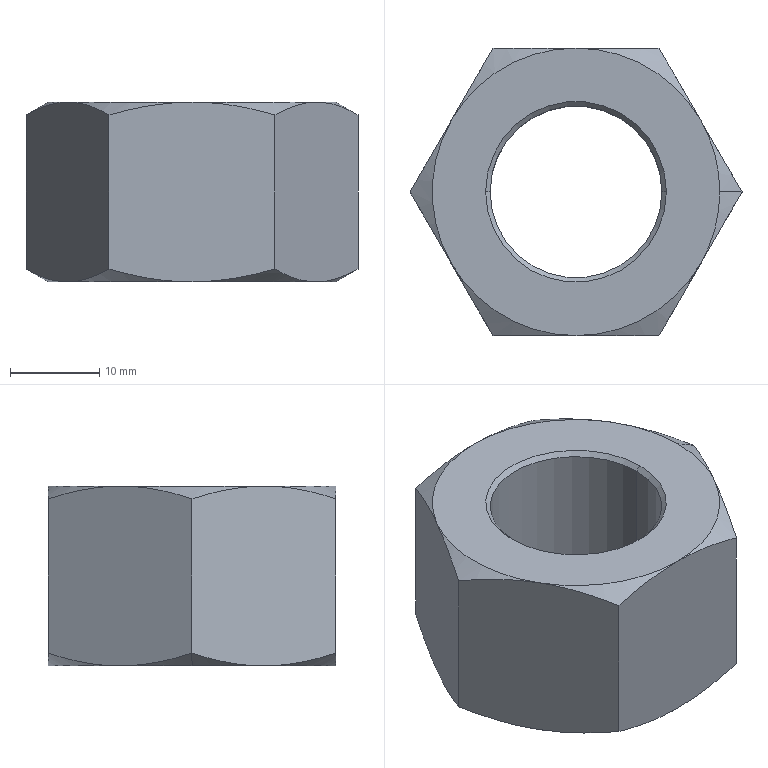Part | SolidWorks | features Cut 2, Chamfer 1, Extrusion 1 | 1 solid | 28 faces | box 37.3 x 32.303 x 20.2 mm | volume 12259 mm3 | cone 18 | plane 8 | cylinder 2 | commonest cylinder face diameters 19.294 x2
STEP:
#1=CARTESIAN_POINT('',(-9.647,0.,19.695));
#2=VERTEX_POINT('',#1);
#3=CARTESIAN_POINT('',(9.647,0.,19.695));
#4=VERTEX_POINT('',#3);
#5=CARTESIAN_POINT('',(0.,0.,19.695));
#6=DIRECTION('',(0.,0.,1.));
#7=DIRECTION('',(-1.,0.,0.));
#8=AXIS2_PLACEMENT_3D('',#5,#6,#7);
#9=CIRCLE('',#8,9.647);
#10=EDGE_CURVE('',#2,#4,#9,.T.);
#11=ORIENTED_EDGE('',*,*,#10,.F.);
#12=CARTESIAN_POINT('',(-10.152,0.,20.2));
#13=VERTEX_POINT('',#12);
#14=CARTESIAN_POINT('',(-9.647,0.,19.695));
#15=DIRECTION('',(-0.7071,0.,0.7071));
#16=VECTOR('',#15,1000.);
#17=LINE('',#14,#16);
#18=EDGE_CURVE('',#2,#13,#17,.T.);
#19=ORIENTED_EDGE('',*,*,#18,.T.);
#20=CARTESIAN_POINT('',(10.152,0.,20.2));
#21=VERTEX_POINT('',#20);
#22=CARTESIAN_POINT('',(0.,0.,20.2));
#23=DIRECTION('',(0.,0.,-1.));
#24=DIRECTION('',(-1.,0.,0.));
#25=AXIS2_PLACEMENT_3D('',#22,#23,#24);
#26=CIRCLE('',#25,10.152);
#27=EDGE_CURVE('',#21,#13,#26,.T.);
#28=ORIENTED_EDGE('',*,*,#27,.F.);
#29=CARTESIAN_POINT('',(9.647,0.,19.695));
#30=DIRECTION('',(0.7071,0.,0.7071));
#31=VECTOR('',#30,1000.);
#32=LINE('',#29,#31);
#33=EDGE_CURVE('',#4,#21,#32,.T.);
#34=ORIENTED_EDGE('',*,*,#33,.F.);
#35=EDGE_LOOP('',(#11,#19,#28,#34));
#36=FACE_OUTER_BOUND('',#35,.T.);
#37=CARTESIAN_POINT('',(0.,0.,19.695));
#38=DIRECTION('',(0.,0.,1.));
#39=DIRECTION('',(1.,0.,0.));
#40=AXIS2_PLACEMENT_3D('',#37,#38,#39);
#41=CONICAL_SURFACE('',#40,9.647,0.7854);
#42=ADVANCED_FACE('',(#36),#41,.F.);
#43=CARTESIAN_POINT('',(9.647,0.,0.505));
#44=VERTEX_POINT('',#43);
#45=CARTESIAN_POINT('',(-9.647,0.,0.505));
#46=VERTEX_POINT('',#45);
#47=CARTESIAN_POINT('',(0.,0.,0.505));
#48=DIRECTION('',(0.,0.,-1.));
#49=DIRECTION('',(-1.,0.,0.));
#50=AXIS2_PLACEMENT_3D('',#47,#48,#49);
#51=CIRCLE('',#50,9.647);
#52=EDGE_CURVE('',#44,#46,#51,.T.);
#53=ORIENTED_EDGE('',*,*,#52,.F.);
#54=CARTESIAN_POINT('',(10.152,0.,0.));
#55=VERTEX_POINT('',#54);
#56=CARTESIAN_POINT('',(10.152,0.,0.));
#57=DIRECTION('',(0.7071,0.,-0.7071));
#58=VECTOR('',#57,1000.);
#59=LINE('',#56,#58);
#60=EDGE_CURVE('',#44,#55,#59,.T.);
#61=ORIENTED_EDGE('',*,*,#60,.T.);
#62=CARTESIAN_POINT('',(-10.152,0.,0.));
#63=VERTEX_POINT('',#62);
#64=CARTESIAN_POINT('',(0.,0.,0.));
#65=DIRECTION('',(0.,0.,1.));
#66=DIRECTION('',(-1.,0.,0.));
#67=AXIS2_PLACEMENT_3D('',#64,#65,#66);
#68=CIRCLE('',#67,10.152);
#69=EDGE_CURVE('',#63,#55,#68,.T.);
#70=ORIENTED_EDGE('',*,*,#69,.F.);
#71=CARTESIAN_POINT('',(-10.152,0.,0.));
#72=DIRECTION('',(-0.7071,0.,-0.7071));
#73=VECTOR('',#72,1000.);
#74=LINE('',#71,#73);
#75=EDGE_CURVE('',#46,#63,#74,.T.);
#76=ORIENTED_EDGE('',*,*,#75,.F.);
#77=EDGE_LOOP('',(#53,#61,#70,#76));
#78=FACE_OUTER_BOUND('',#77,.T.);
#79=CARTESIAN_POINT('',(0.,0.,0.));
#80=DIRECTION('',(0.,0.,-1.));
#81=DIRECTION('',(-1.,0.,0.));
#82=AXIS2_PLACEMENT_3D('',#79,#80,#81);
#83=CONICAL_SURFACE('',#82,10.152,0.7854);
#84=ADVANCED_FACE('',(#78),#83,.F.);
#85=CARTESIAN_POINT('',(13.988,8.076,20.2));
#86=VERTEX_POINT('',#85);
#87=CARTESIAN_POINT('',(16.151,0.,20.2));
#88=VERTEX_POINT('',#87);
#89=CARTESIAN_POINT('',(0.,0.,20.2));
#90=DIRECTION('',(0.,0.,-1.));
#91=DIRECTION('',(-1.,0.,0.));
#92=AXIS2_PLACEMENT_3D('',#89,#90,#91);
#93=CIRCLE('',#92,16.151);
#94=EDGE_CURVE('',#86,#88,#93,.T.);
#95=ORIENTED_EDGE('',*,*,#94,.T.);
#96=CARTESIAN_POINT('',(18.65,0.,18.757));
#97=VERTEX_POINT('',#96);
#98=CARTESIAN_POINT('',(16.151,0.,20.2));
#99=DIRECTION('',(0.866,0.,-0.5));
#100=VECTOR('',#99,1000.);
#101=LINE('',#98,#100);
#102=EDGE_CURVE('',#88,#97,#101,.T.);
#103=ORIENTED_EDGE('',*,*,#102,.T.);
#104=CARTESIAN_POINT('',(18.65,0.,18.757));
#105=CARTESIAN_POINT('',(17.887,1.321,19.198));
#106=CARTESIAN_POINT('',(17.119,2.652,19.561));
#107=CARTESIAN_POINT('',(15.566,5.341,20.063));
#108=CARTESIAN_POINT('',(14.782,6.7,20.2));
#109=CARTESIAN_POINT('',(13.988,8.076,20.2));
#110=B_SPLINE_CURVE_WITH_KNOTS('',3,(#104,#105,#106,#107,#108,#109),.UNSPECIFIED.,.F.,.F.,(4,2,4),(0.000000238,0.004718,0.009436),.UNSPECIFIED.);
#111=EDGE_CURVE('',#97,#86,#110,.T.);
#112=ORIENTED_EDGE('',*,*,#111,.T.);
#113=EDGE_LOOP('',(#95,#103,#112));
#114=FACE_OUTER_BOUND('',#113,.T.);
#115=CARTESIAN_POINT('',(0.,0.,20.2));
#116=DIRECTION('',(0.,0.,-1.));
#117=DIRECTION('',(1.,0.,0.));
#118=AXIS2_PLACEMENT_3D('',#115,#116,#117);
#119=CONICAL_SURFACE('',#118,16.151,1.047);
#120=ADVANCED_FACE('',(#114),#119,.T.);
#121=CARTESIAN_POINT('',(-16.151,0.,0.));
#122=VERTEX_POINT('',#121);
#123=CARTESIAN_POINT('',(-13.988,8.076,0.));
#124=VERTEX_POINT('',#123);
#125=CARTESIAN_POINT('',(0.,0.,0.));
#126=DIRECTION('',(0.,0.,-1.));
#127=DIRECTION('',(-1.,0.,0.));
#128=AXIS2_PLACEMENT_3D('',#125,#126,#127);
#129=CIRCLE('',#128,16.151);
#130=EDGE_CURVE('',#122,#124,#129,.T.);
#131=ORIENTED_EDGE('',*,*,#130,.F.);
#132=CARTESIAN_POINT('',(-18.65,0.,1.443));
#133=VERTEX_POINT('',#132);
#134=CARTESIAN_POINT('',(-16.151,0.,0.));
#135=DIRECTION('',(-0.866,0.,0.5));
#136=VECTOR('',#135,1000.);
#137=LINE('',#134,#136);
#138=EDGE_CURVE('',#122,#133,#137,.T.);
#139=ORIENTED_EDGE('',*,*,#138,.T.);
#140=CARTESIAN_POINT('',(-18.65,0.,1.443));
#141=CARTESIAN_POINT('',(-17.887,1.321,1.002));
#142=CARTESIAN_POINT('',(-17.119,2.652,0.6394));
#143=CARTESIAN_POINT('',(-15.566,5.341,0.1375));
#144=CARTESIAN_POINT('',(-14.782,6.7,0.));
#145=CARTESIAN_POINT('',(-13.988,8.076,0.));
#146=B_SPLINE_CURVE_WITH_KNOTS('',3,(#140,#141,#142,#143,#144,#145),.UNSPECIFIED.,.F.,.F.,(4,2,4),(0.000000238,0.004718,0.009436),.UNSPECIFIED.);
#147=EDGE_CURVE('',#133,#124,#146,.T.);
#148=ORIENTED_EDGE('',*,*,#147,.T.);
#149=EDGE_LOOP('',(#131,#139,#148));
#150=FACE_OUTER_BOUND('',#149,.T.);
#151=CARTESIAN_POINT('',(0.,0.,0.));
#152=DIRECTION('',(0.,0.,1.));
#153=DIRECTION('',(-1.,0.,0.));
#154=AXIS2_PLACEMENT_3D('',#151,#152,#153);
#155=CONICAL_SURFACE('',#154,16.151,1.047);
#156=ADVANCED_FACE('',(#150),#155,.T.);
#157=ORIENTED_EDGE('',*,*,#10,.T.);
#158=CARTESIAN_POINT('',(9.647,0.,20.2));
#159=DIRECTION('',(0.,0.,-1.));
#160=VECTOR('',#159,1000.);
#161=LINE('',#158,#160);
#162=EDGE_CURVE('',#4,#44,#161,.T.);
#163=ORIENTED_EDGE('',*,*,#162,.T.);
#164=ORIENTED_EDGE('',*,*,#52,.T.);
#165=CARTESIAN_POINT('',(-9.647,0.,20.2));
#166=DIRECTION('',(0.,0.,-1.));
#167=VECTOR('',#166,1000.);
#168=LINE('',#165,#167);
#169=EDGE_CURVE('',#2,#46,#168,.T.);
#170=ORIENTED_EDGE('',*,*,#169,.F.);
#171=EDGE_LOOP('',(#157,#163,#164,#170));
#172=FACE_OUTER_BOUND('',#171,.T.);
#173=CARTESIAN_POINT('',(0.,0.,20.2));
#174=DIRECTION('',(0.,0.,-1.));
#175=DIRECTION('',(-1.,0.,0.));
#176=AXIS2_PLACEMENT_3D('',#173,#174,#175);
#177=CYLINDRICAL_SURFACE('',#176,9.647);
#178=ADVANCED_FACE('',(#172),#177,.F.);
#179=ORIENTED_EDGE('',*,*,#111,.F.);
#180=CARTESIAN_POINT('',(18.65,0.,1.443));
#181=VERTEX_POINT('',#180);
#182=CARTESIAN_POINT('',(18.65,0.,20.2));
#183=DIRECTION('',(0.,0.,-1.));
#184=VECTOR('',#183,1000.);
#185=LINE('',#182,#184);
#186=EDGE_CURVE('',#97,#181,#185,.T.);
#187=ORIENTED_EDGE('',*,*,#186,.T.);
#188=CARTESIAN_POINT('',(13.988,8.076,0.));
#189=VERTEX_POINT('',#188);
#190=CARTESIAN_POINT('',(13.988,8.076,0.));
#191=CARTESIAN_POINT('',(14.383,7.39,0.));
#192=CARTESIAN_POINT('',(14.781,6.702,0.0341));
#193=CARTESIAN_POINT('',(15.567,5.34,0.166));
#194=CARTESIAN_POINT('',(15.957,4.664,0.2638));
#195=CARTESIAN_POINT('',(17.122,2.647,0.6407));
#196=CARTESIAN_POINT('',(17.889,1.318,1.003));
#197=CARTESIAN_POINT('',(18.65,0.,1.443));
#198=B_SPLINE_CURVE_WITH_KNOTS('',3,(#190,#191,#192,#193,#194,#195,#196,#197),.UNSPECIFIED.,.F.,.F.,(4,2,2,4),(0.009436,0.01179,0.01414,0.01884),.UNSPECIFIED.);
#199=EDGE_CURVE('',#189,#181,#198,.T.);
#200=ORIENTED_EDGE('',*,*,#199,.F.);
#201=CARTESIAN_POINT('',(9.325,16.151,1.443));
#202=VERTEX_POINT('',#201);
#203=CARTESIAN_POINT('',(9.325,16.151,1.443));
#204=CARTESIAN_POINT('',(10.088,14.83,1.002));
#205=CARTESIAN_POINT('',(10.856,13.5,0.6394));
#206=CARTESIAN_POINT('',(12.409,10.81,0.1375));
#207=CARTESIAN_POINT('',(13.193,9.452,0.));
#208=CARTESIAN_POINT('',(13.988,8.076,0.));
#209=B_SPLINE_CURVE_WITH_KNOTS('',3,(#203,#204,#205,#206,#207,#208),.UNSPECIFIED.,.F.,.F.,(4,2,4),(0.000000238,0.004718,0.009436),.UNSPECIFIED.);
#210=EDGE_CURVE('',#202,#189,#209,.T.);
#211=ORIENTED_EDGE('',*,*,#210,.F.);
#212=CARTESIAN_POINT('',(9.325,16.151,18.757));
#213=VERTEX_POINT('',#212);
#214=CARTESIAN_POINT('',(9.325,16.151,20.2));
#215=DIRECTION('',(0.,0.,-1.));
#216=VECTOR('',#215,1000.);
#217=LINE('',#214,#216);
#218=EDGE_CURVE('',#213,#202,#217,.T.);
#219=ORIENTED_EDGE('',*,*,#218,.F.);
#220=CARTESIAN_POINT('',(13.988,8.076,20.2));
#221=CARTESIAN_POINT('',(13.592,8.761,20.2));
#222=CARTESIAN_POINT('',(13.194,9.449,20.166));
#223=CARTESIAN_POINT('',(12.408,10.811,20.034));
#224=CARTESIAN_POINT('',(12.018,11.488,19.936));
#225=CARTESIAN_POINT('',(10.853,13.505,19.559));
#226=CARTESIAN_POINT('',(10.086,14.834,19.197));
#227=CARTESIAN_POINT('',(9.325,16.151,18.757));
#228=B_SPLINE_CURVE_WITH_KNOTS('',3,(#220,#221,#222,#223,#224,#225,#226,#227),.UNSPECIFIED.,.F.,.F.,(4,2,2,4),(0.009436,0.01179,0.01414,0.01884),.UNSPECIFIED.);
#229=EDGE_CURVE('',#86,#213,#228,.T.);
#230=ORIENTED_EDGE('',*,*,#229,.F.);
#231=EDGE_LOOP('',(#179,#187,#200,#211,#219,#230));
#232=FACE_OUTER_BOUND('',#231,.T.);
#233=CARTESIAN_POINT('',(18.65,0.,20.2));
#234=DIRECTION('',(-0.866,-0.5,0.));
#235=DIRECTION('',(0.5,-0.866,0.));
#236=AXIS2_PLACEMENT_3D('',#233,#234,#235);
#237=PLANE('',#236);
#238=ADVANCED_FACE('',(#232),#237,.F.);
#239=CARTESIAN_POINT('',(0.,16.151,20.2));
#240=VERTEX_POINT('',#239);
#241=CARTESIAN_POINT('',(9.325,16.151,18.757));
#242=CARTESIAN_POINT('',(7.817,16.151,19.193));
#243=CARTESIAN_POINT('',(6.29,16.151,19.555));
#244=CARTESIAN_POINT('',(3.955,16.151,19.934));
#245=CARTESIAN_POINT('',(3.17,16.151,20.033));
#246=CARTESIAN_POINT('',(1.582,16.151,20.166));
#247=CARTESIAN_POINT('',(0.7891,16.151,20.2));
#248=CARTESIAN_POINT('',(0.,16.151,20.2));
#249=B_SPLINE_CURVE_WITH_KNOTS('',3,(#241,#242,#243,#244,#245,#246,#247,#248),.UNSPECIFIED.,.F.,.F.,(4,2,2,4),(0.05347,0.05819,0.06055,0.06291),.UNSPECIFIED.);
#250=EDGE_CURVE('',#213,#240,#249,.T.);
#251=ORIENTED_EDGE('',*,*,#250,.F.);
#252=ORIENTED_EDGE('',*,*,#218,.T.);
#253=CARTESIAN_POINT('',(0.,16.151,0.));
#254=VERTEX_POINT('',#253);
#255=CARTESIAN_POINT('',(0.,16.151,0.));
#256=CARTESIAN_POINT('',(0.7891,16.151,0.));
#257=CARTESIAN_POINT('',(1.582,16.151,0.03365));
#258=CARTESIAN_POINT('',(3.17,16.151,0.1671));
#259=CARTESIAN_POINT('',(3.955,16.151,0.2658));
#260=CARTESIAN_POINT('',(6.29,16.151,0.6449));
#261=CARTESIAN_POINT('',(7.817,16.151,1.007));
#262=CARTESIAN_POINT('',(9.325,16.151,1.443));
#263=B_SPLINE_CURVE_WITH_KNOTS('',3,(#255,#256,#257,#258,#259,#260,#261,#262),.UNSPECIFIED.,.F.,.F.,(4,2,2,4),(0.02654,0.0289,0.03126,0.03599),.UNSPECIFIED.);
#264=EDGE_CURVE('',#254,#202,#263,.T.);
#265=ORIENTED_EDGE('',*,*,#264,.F.);
#266=CARTESIAN_POINT('',(-9.325,16.151,1.443));
#267=VERTEX_POINT('',#266);
#268=CARTESIAN_POINT('',(-9.325,16.151,1.443));
#269=CARTESIAN_POINT('',(-8.566,16.151,1.223));
#270=CARTESIAN_POINT('',(-7.799,16.151,1.022));
#271=CARTESIAN_POINT('',(-6.252,16.151,0.6658));
#272=CARTESIAN_POINT('',(-5.476,16.151,0.512));
#273=CARTESIAN_POINT('',(-3.143,16.151,0.1357));
#274=CARTESIAN_POINT('',(-1.577,16.151,0.));
#275=CARTESIAN_POINT('',(0.,16.151,0.));
#276=B_SPLINE_CURVE_WITH_KNOTS('',3,(#268,#269,#270,#271,#272,#273,#274,#275),.UNSPECIFIED.,.F.,.F.,(4,2,2,4),(0.0171,0.01946,0.02182,0.02654),.UNSPECIFIED.);
#277=EDGE_CURVE('',#267,#254,#276,.T.);
#278=ORIENTED_EDGE('',*,*,#277,.F.);
#279=CARTESIAN_POINT('',(-9.325,16.151,18.757));
#280=VERTEX_POINT('',#279);
#281=CARTESIAN_POINT('',(-9.325,16.151,20.2));
#282=DIRECTION('',(0.,0.,-1.));
#283=VECTOR('',#282,1000.);
#284=LINE('',#281,#283);
#285=EDGE_CURVE('',#280,#267,#284,.T.);
#286=ORIENTED_EDGE('',*,*,#285,.F.);
#287=CARTESIAN_POINT('',(0.,16.151,20.2));
#288=CARTESIAN_POINT('',(-1.577,16.151,20.2));
#289=CARTESIAN_POINT('',(-3.143,16.151,20.064));
#290=CARTESIAN_POINT('',(-5.476,16.151,19.688));
#291=CARTESIAN_POINT('',(-6.252,16.151,19.534));
#292=CARTESIAN_POINT('',(-7.799,16.151,19.178));
#293=CARTESIAN_POINT('',(-8.566,16.151,18.977));
#294=CARTESIAN_POINT('',(-9.325,16.151,18.757));
#295=B_SPLINE_CURVE_WITH_KNOTS('',3,(#287,#288,#289,#290,#291,#292,#293,#294),.UNSPECIFIED.,.F.,.F.,(4,2,2,4),(0.06291,0.06763,0.06999,0.07235),.UNSPECIFIED.);
#296=EDGE_CURVE('',#240,#280,#295,.T.);
#297=ORIENTED_EDGE('',*,*,#296,.F.);
#298=EDGE_LOOP('',(#251,#252,#265,#278,#286,#297));
#299=FACE_OUTER_BOUND('',#298,.T.);
#300=CARTESIAN_POINT('',(9.325,16.151,20.2));
#301=DIRECTION('',(0.,-1.,0.));
#302=DIRECTION('',(1.,0.,0.));
#303=AXIS2_PLACEMENT_3D('',#300,#301,#302);
#304=PLANE('',#303);
#305=ADVANCED_FACE('',(#299),#304,.F.);
#306=CARTESIAN_POINT('',(-13.988,8.076,20.2));
#307=VERTEX_POINT('',#306);
#308=CARTESIAN_POINT('',(-9.325,16.151,18.757));
#309=CARTESIAN_POINT('',(-10.088,14.83,19.198));
#310=CARTESIAN_POINT('',(-10.856,13.5,19.561));
#311=CARTESIAN_POINT('',(-12.409,10.81,20.063));
#312=CARTESIAN_POINT('',(-13.193,9.452,20.2));
#313=CARTESIAN_POINT('',(-13.988,8.076,20.2));
#314=B_SPLINE_CURVE_WITH_KNOTS('',3,(#308,#309,#310,#311,#312,#313),.UNSPECIFIED.,.F.,.F.,(4,2,4),(0.000000238,0.004718,0.009436),.UNSPECIFIED.);
#315=EDGE_CURVE('',#280,#307,#314,.T.);
#316=ORIENTED_EDGE('',*,*,#315,.F.);
#317=ORIENTED_EDGE('',*,*,#285,.T.);
#318=CARTESIAN_POINT('',(-13.988,8.076,0.));
#319=CARTESIAN_POINT('',(-13.592,8.761,0.));
#320=CARTESIAN_POINT('',(-13.194,9.449,0.0341));
#321=CARTESIAN_POINT('',(-12.408,10.811,0.166));
#322=CARTESIAN_POINT('',(-12.018,11.488,0.2638));
#323=CARTESIAN_POINT('',(-10.853,13.505,0.6407));
#324=CARTESIAN_POINT('',(-10.086,14.834,1.003));
#325=CARTESIAN_POINT('',(-9.325,16.151,1.443));
#326=B_SPLINE_CURVE_WITH_KNOTS('',3,(#318,#319,#320,#321,#322,#323,#324,#325),.UNSPECIFIED.,.F.,.F.,(4,2,2,4),(0.009436,0.01179,0.01414,0.01884),.UNSPECIFIED.);
#327=EDGE_CURVE('',#124,#267,#326,.T.);
#328=ORIENTED_EDGE('',*,*,#327,.F.);
#329=ORIENTED_EDGE('',*,*,#147,.F.);
#330=CARTESIAN_POINT('',(-18.65,0.,18.757));
#331=VERTEX_POINT('',#330);
#332=CARTESIAN_POINT('',(-18.65,0.,20.2));
#333=DIRECTION('',(0.,0.,-1.));
#334=VECTOR('',#333,1000.);
#335=LINE('',#332,#334);
#336=EDGE_CURVE('',#331,#133,#335,.T.);
#337=ORIENTED_EDGE('',*,*,#336,.F.);
#338=CARTESIAN_POINT('',(-13.988,8.076,20.2));
#339=CARTESIAN_POINT('',(-14.383,7.39,20.2));
#340=CARTESIAN_POINT('',(-14.781,6.702,20.166));
#341=CARTESIAN_POINT('',(-15.567,5.34,20.034));
#342=CARTESIAN_POINT('',(-15.957,4.664,19.936));
#343=CARTESIAN_POINT('',(-17.122,2.647,19.559));
#344=CARTESIAN_POINT('',(-17.889,1.318,19.197));
#345=CARTESIAN_POINT('',(-18.65,0.,18.757));
#346=B_SPLINE_CURVE_WITH_KNOTS('',3,(#338,#339,#340,#341,#342,#343,#344,#345),.UNSPECIFIED.,.F.,.F.,(4,2,2,4),(0.009436,0.01179,0.01414,0.01884),.UNSPECIFIED.);
#347=EDGE_CURVE('',#307,#331,#346,.T.);
#348=ORIENTED_EDGE('',*,*,#347,.F.);
#349=EDGE_LOOP('',(#316,#317,#328,#329,#337,#348));
#350=FACE_OUTER_BOUND('',#349,.T.);
#351=CARTESIAN_POINT('',(-9.325,16.151,20.2));
#352=DIRECTION('',(0.866,-0.5,0.));
#353=DIRECTION('',(0.5,0.866,0.));
#354=AXIS2_PLACEMENT_3D('',#351,#352,#353);
#355=PLANE('',#354);
#356=ADVANCED_FACE('',(#350),#355,.F.);
#357=CARTESIAN_POINT('',(-13.988,-8.076,20.2));
#358=VERTEX_POINT('',#357);
#359=CARTESIAN_POINT('',(-18.65,0.,18.757));
#360=CARTESIAN_POINT('',(-17.887,-1.321,19.198));
#361=CARTESIAN_POINT('',(-17.119,-2.652,19.561));
#362=CARTESIAN_POINT('',(-15.566,-5.341,20.063));
#363=CARTESIAN_POINT('',(-14.782,-6.7,20.2));
#364=CARTESIAN_POINT('',(-13.988,-8.076,20.2));
#365=B_SPLINE_CURVE_WITH_KNOTS('',3,(#359,#360,#361,#362,#363,#364),.UNSPECIFIED.,.F.,.F.,(4,2,4),(0.000000238,0.004718,0.009436),.UNSPECIFIED.);
#366=EDGE_CURVE('',#331,#358,#365,.T.);
#367=ORIENTED_EDGE('',*,*,#366,.F.);
#368=ORIENTED_EDGE('',*,*,#336,.T.);
#369=CARTESIAN_POINT('',(-13.987,-8.076,0.));
#370=VERTEX_POINT('',#369);
#371=CARTESIAN_POINT('',(-13.987,-8.076,0.));
#372=CARTESIAN_POINT('',(-14.383,-7.39,0.));
#373=CARTESIAN_POINT('',(-14.781,-6.702,0.0341));
#374=CARTESIAN_POINT('',(-15.567,-5.34,0.166));
#375=CARTESIAN_POINT('',(-15.957,-4.664,0.2638));
#376=CARTESIAN_POINT('',(-17.122,-2.647,0.6407));
#377=CARTESIAN_POINT('',(-17.889,-1.318,1.003));
#378=CARTESIAN_POINT('',(-18.65,0.,1.443));
#379=B_SPLINE_CURVE_WITH_KNOTS('',3,(#371,#372,#373,#374,#375,#376,#377,#378),.UNSPECIFIED.,.F.,.F.,(4,2,2,4),(0.009436,0.01179,0.01414,0.01884),.UNSPECIFIED.);
#380=EDGE_CURVE('',#370,#133,#379,.T.);
#381=ORIENTED_EDGE('',*,*,#380,.F.);
#382=CARTESIAN_POINT('',(-9.325,-16.151,1.443));
#383=VERTEX_POINT('',#382);
#384=CARTESIAN_POINT('',(-9.325,-16.151,1.443));
#385=CARTESIAN_POINT('',(-10.088,-14.83,1.002));
#386=CARTESIAN_POINT('',(-10.856,-13.5,0.6394));
#387=CARTESIAN_POINT('',(-12.409,-10.81,0.1375));
#388=CARTESIAN_POINT('',(-13.193,-9.452,0.));
#389=CARTESIAN_POINT('',(-13.987,-8.076,0.));
#390=B_SPLINE_CURVE_WITH_KNOTS('',3,(#384,#385,#386,#387,#388,#389),.UNSPECIFIED.,.F.,.F.,(4,2,4),(0.000000238,0.004718,0.009436),.UNSPECIFIED.);
#391=EDGE_CURVE('',#383,#370,#390,.T.);
#392=ORIENTED_EDGE('',*,*,#391,.F.);
#393=CARTESIAN_POINT('',(-9.325,-16.151,18.757));
#394=VERTEX_POINT('',#393);
#395=CARTESIAN_POINT('',(-9.325,-16.151,20.2));
#396=DIRECTION('',(0.,0.,-1.));
#397=VECTOR('',#396,1000.);
#398=LINE('',#395,#397);
#399=EDGE_CURVE('',#394,#383,#398,.T.);
#400=ORIENTED_EDGE('',*,*,#399,.F.);
#401=CARTESIAN_POINT('',(-13.988,-8.076,20.2));
#402=CARTESIAN_POINT('',(-13.592,-8.761,20.2));
#403=CARTESIAN_POINT('',(-13.194,-9.449,20.166));
#404=CARTESIAN_POINT('',(-12.408,-10.811,20.034));
#405=CARTESIAN_POINT('',(-12.018,-11.488,19.936));
#406=CARTESIAN_POINT('',(-10.853,-13.505,19.559));
#407=CARTESIAN_POINT('',(-10.086,-14.834,19.197));
#408=CARTESIAN_POINT('',(-9.325,-16.151,18.757));
#409=B_SPLINE_CURVE_WITH_KNOTS('',3,(#401,#402,#403,#404,#405,#406,#407,#408),.UNSPECIFIED.,.F.,.F.,(4,2,2,4),(0.009436,0.01179,0.01414,0.01884),.UNSPECIFIED.);
#410=EDGE_CURVE('',#358,#394,#409,.T.);
#411=ORIENTED_EDGE('',*,*,#410,.F.);
#412=EDGE_LOOP('',(#367,#368,#381,#392,#400,#411));
#413=FACE_OUTER_BOUND('',#412,.T.);
#414=CARTESIAN_POINT('',(-18.65,0.,20.2));
#415=DIRECTION('',(0.866,0.5,0.));
#416=DIRECTION('',(-0.5,0.866,0.));
#417=AXIS2_PLACEMENT_3D('',#414,#415,#416);
#418=PLANE('',#417);
#419=ADVANCED_FACE('',(#413),#418,.F.);
#420=CARTESIAN_POINT('',(0.,-16.151,20.2));
#421=VERTEX_POINT('',#420);
#422=CARTESIAN_POINT('',(-9.325,-16.151,18.757));
#423=CARTESIAN_POINT('',(-8.566,-16.151,18.977));
#424=CARTESIAN_POINT('',(-7.799,-16.151,19.178));
#425=CARTESIAN_POINT('',(-6.252,-16.151,19.534));
#426=CARTESIAN_POINT('',(-5.476,-16.151,19.688));
#427=CARTESIAN_POINT('',(-3.143,-16.151,20.064));
#428=CARTESIAN_POINT('',(-1.577,-16.151,20.2));
#429=CARTESIAN_POINT('',(0.,-16.151,20.2));
#430=B_SPLINE_CURVE_WITH_KNOTS('',3,(#422,#423,#424,#425,#426,#427,#428,#429),.UNSPECIFIED.,.F.,.F.,(4,2,2,4),(0.0171,0.01946,0.02182,0.02654),.UNSPECIFIED.);
#431=EDGE_CURVE('',#394,#421,#430,.T.);
#432=ORIENTED_EDGE('',*,*,#431,.F.);
#433=ORIENTED_EDGE('',*,*,#399,.T.);
#434=CARTESIAN_POINT('',(0.,-16.151,0.));
#435=VERTEX_POINT('',#434);
#436=CARTESIAN_POINT('',(0.,-16.151,0.));
#437=CARTESIAN_POINT('',(-1.577,-16.151,0.));
#438=CARTESIAN_POINT('',(-3.143,-16.151,0.1357));
#439=CARTESIAN_POINT('',(-5.476,-16.151,0.512));
#440=CARTESIAN_POINT('',(-6.252,-16.151,0.6658));
#441=CARTESIAN_POINT('',(-7.799,-16.151,1.022));
#442=CARTESIAN_POINT('',(-8.566,-16.151,1.223));
#443=CARTESIAN_POINT('',(-9.325,-16.151,1.443));
#444=B_SPLINE_CURVE_WITH_KNOTS('',3,(#436,#437,#438,#439,#440,#441,#442,#443),.UNSPECIFIED.,.F.,.F.,(4,2,2,4),(0.06291,0.06763,0.06999,0.07235),.UNSPECIFIED.);
#445=EDGE_CURVE('',#435,#383,#444,.T.);
#446=ORIENTED_EDGE('',*,*,#445,.F.);
#447=CARTESIAN_POINT('',(9.325,-16.151,1.443));
#448=VERTEX_POINT('',#447);
#449=CARTESIAN_POINT('',(9.325,-16.151,1.443));
#450=CARTESIAN_POINT('',(7.817,-16.151,1.007));
#451=CARTESIAN_POINT('',(6.29,-16.151,0.6449));
#452=CARTESIAN_POINT('',(3.955,-16.151,0.2658));
#453=CARTESIAN_POINT('',(3.17,-16.151,0.1671));
#454=CARTESIAN_POINT('',(1.582,-16.151,0.03365));
#455=CARTESIAN_POINT('',(0.7891,-16.151,0.));
#456=CARTESIAN_POINT('',(0.,-16.151,0.));
#457=B_SPLINE_CURVE_WITH_KNOTS('',3,(#449,#450,#451,#452,#453,#454,#455,#456),.UNSPECIFIED.,.F.,.F.,(4,2,2,4),(0.05347,0.05819,0.06055,0.06291),.UNSPECIFIED.);
#458=EDGE_CURVE('',#448,#435,#457,.T.);
#459=ORIENTED_EDGE('',*,*,#458,.F.);
#460=CARTESIAN_POINT('',(9.325,-16.151,18.757));
#461=VERTEX_POINT('',#460);
#462=CARTESIAN_POINT('',(9.325,-16.151,20.2));
#463=DIRECTION('',(0.,0.,-1.));
#464=VECTOR('',#463,1000.);
#465=LINE('',#462,#464);
#466=EDGE_CURVE('',#461,#448,#465,.T.);
#467=ORIENTED_EDGE('',*,*,#466,.F.);
#468=CARTESIAN_POINT('',(0.,-16.151,20.2));
#469=CARTESIAN_POINT('',(0.7891,-16.151,20.2));
#470=CARTESIAN_POINT('',(1.582,-16.151,20.166));
#471=CARTESIAN_POINT('',(3.17,-16.151,20.033));
#472=CARTESIAN_POINT('',(3.955,-16.151,19.934));
#473=CARTESIAN_POINT('',(6.29,-16.151,19.555));
#474=CARTESIAN_POINT('',(7.817,-16.151,19.193));
#475=CARTESIAN_POINT('',(9.325,-16.151,18.757));
#476=B_SPLINE_CURVE_WITH_KNOTS('',3,(#468,#469,#470,#471,#472,#473,#474,#475),.UNSPECIFIED.,.F.,.F.,(4,2,2,4),(0.02654,0.0289,0.03126,0.03599),.UNSPECIFIED.);
#477=EDGE_CURVE('',#421,#461,#476,.T.);
#478=ORIENTED_EDGE('',*,*,#477,.F.);
#479=EDGE_LOOP('',(#432,#433,#446,#459,#467,#478));
#480=FACE_OUTER_BOUND('',#479,.T.);
#481=CARTESIAN_POINT('',(-9.325,-16.151,20.2));
#482=DIRECTION('',(0.,1.,0.));
#483=DIRECTION('',(-1.,0.,0.));
#484=AXIS2_PLACEMENT_3D('',#481,#482,#483);
#485=PLANE('',#484);
#486=ADVANCED_FACE('',(#480),#485,.F.);
#487=CARTESIAN_POINT('',(13.987,-8.076,20.2));
#488=VERTEX_POINT('',#487);
#489=CARTESIAN_POINT('',(9.325,-16.151,18.757));
#490=CARTESIAN_POINT('',(10.088,-14.83,19.198));
#491=CARTESIAN_POINT('',(10.856,-13.5,19.561));
#492=CARTESIAN_POINT('',(12.409,-10.81,20.063));
#493=CARTESIAN_POINT('',(13.193,-9.452,20.2));
#494=CARTESIAN_POINT('',(13.987,-8.076,20.2));
#495=B_SPLINE_CURVE_WITH_KNOTS('',3,(#489,#490,#491,#492,#493,#494),.UNSPECIFIED.,.F.,.F.,(4,2,4),(0.000000238,0.004718,0.009436),.UNSPECIFIED.);
#496=EDGE_CURVE('',#461,#488,#495,.T.);
#497=ORIENTED_EDGE('',*,*,#496,.F.);
#498=ORIENTED_EDGE('',*,*,#466,.T.);
#499=CARTESIAN_POINT('',(13.987,-8.076,0.));
#500=VERTEX_POINT('',#499);
#501=CARTESIAN_POINT('',(13.987,-8.076,0.));
#502=CARTESIAN_POINT('',(13.592,-8.761,0.));
#503=CARTESIAN_POINT('',(13.194,-9.449,0.0341));
#504=CARTESIAN_POINT('',(12.408,-10.811,0.166));
#505=CARTESIAN_POINT('',(12.018,-11.488,0.2638));
#506=CARTESIAN_POINT('',(10.853,-13.505,0.6407));
#507=CARTESIAN_POINT('',(10.086,-14.834,1.003));
#508=CARTESIAN_POINT('',(9.325,-16.151,1.443));
#509=B_SPLINE_CURVE_WITH_KNOTS('',3,(#501,#502,#503,#504,#505,#506,#507,#508),.UNSPECIFIED.,.F.,.F.,(4,2,2,4),(0.009436,0.01179,0.01414,0.01884),.UNSPECIFIED.);
#510=EDGE_CURVE('',#500,#448,#509,.T.);
#511=ORIENTED_EDGE('',*,*,#510,.F.);
#512=CARTESIAN_POINT('',(18.65,0.,1.443));
#513=CARTESIAN_POINT('',(17.887,-1.321,1.002));
#514=CARTESIAN_POINT('',(17.119,-2.652,0.6394));
#515=CARTESIAN_POINT('',(15.566,-5.341,0.1375));
#516=CARTESIAN_POINT('',(14.782,-6.7,0.));
#517=CARTESIAN_POINT('',(13.987,-8.076,0.));
#518=B_SPLINE_CURVE_WITH_KNOTS('',3,(#512,#513,#514,#515,#516,#517),.UNSPECIFIED.,.F.,.F.,(4,2,4),(0.000000238,0.004718,0.009436),.UNSPECIFIED.);
#519=EDGE_CURVE('',#181,#500,#518,.T.);
#520=ORIENTED_EDGE('',*,*,#519,.F.);
#521=ORIENTED_EDGE('',*,*,#186,.F.);
#522=CARTESIAN_POINT('',(13.987,-8.076,20.2));
#523=CARTESIAN_POINT('',(14.383,-7.39,20.2));
#524=CARTESIAN_POINT('',(14.781,-6.702,20.166));
#525=CARTESIAN_POINT('',(15.567,-5.34,20.034));
#526=CARTESIAN_POINT('',(15.957,-4.664,19.936));
#527=CARTESIAN_POINT('',(17.122,-2.647,19.559));
#528=CARTESIAN_POINT('',(17.889,-1.318,19.197));
#529=CARTESIAN_POINT('',(18.65,0.,18.757));
#530=B_SPLINE_CURVE_WITH_KNOTS('',3,(#522,#523,#524,#525,#526,#527,#528,#529),.UNSPECIFIED.,.F.,.F.,(4,2,2,4),(0.009436,0.01179,0.01414,0.01884),.UNSPECIFIED.);
#531=EDGE_CURVE('',#488,#97,#530,.T.);
#532=ORIENTED_EDGE('',*,*,#531,.F.);
#533=EDGE_LOOP('',(#497,#498,#511,#520,#521,#532));
#534=FACE_OUTER_BOUND('',#533,.T.);
#535=CARTESIAN_POINT('',(9.325,-16.151,20.2));
#536=DIRECTION('',(-0.866,0.5,0.));
#537=DIRECTION('',(-0.5,-0.866,0.));
#538=AXIS2_PLACEMENT_3D('',#535,#536,#537);
#539=PLANE('',#538);
#540=ADVANCED_FACE('',(#534),#539,.F.);
#541=ORIENTED_EDGE('',*,*,#27,.T.);
#542=CARTESIAN_POINT('',(0.,0.,20.2));
#543=DIRECTION('',(0.,0.,-1.));
#544=DIRECTION('',(-1.,0.,0.));
#545=AXIS2_PLACEMENT_3D('',#542,#543,#544);
#546=CIRCLE('',#545,10.152);
#547=EDGE_CURVE('',#13,#21,#546,.T.);
#548=ORIENTED_EDGE('',*,*,#547,.T.);
#549=EDGE_LOOP('',(#541,#548));
#550=FACE_BOUND('',#549,.T.);
#551=CARTESIAN_POINT('',(0.,0.,20.2));
#552=DIRECTION('',(0.,0.,-1.));
#553=DIRECTION('',(-1.,0.,0.));
#554=AXIS2_PLACEMENT_3D('',#551,#552,#553);
#555=CIRCLE('',#554,16.151);
#556=EDGE_CURVE('',#307,#240,#555,.T.);
#557=ORIENTED_EDGE('',*,*,#556,.F.);
#558=CARTESIAN_POINT('',(0.,0.,20.2));
#559=DIRECTION('',(0.,0.,-1.));
#560=DIRECTION('',(-1.,0.,0.));
#561=AXIS2_PLACEMENT_3D('',#558,#559,#560);
#562=CIRCLE('',#561,16.151);
#563=EDGE_CURVE('',#358,#307,#562,.T.);
#564=ORIENTED_EDGE('',*,*,#563,.F.);
#565=CARTESIAN_POINT('',(0.,0.,20.2));
#566=DIRECTION('',(0.,0.,-1.));
#567=DIRECTION('',(-1.,0.,0.));
#568=AXIS2_PLACEMENT_3D('',#565,#566,#567);
#569=CIRCLE('',#568,16.151);
#570=EDGE_CURVE('',#421,#358,#569,.T.);
#571=ORIENTED_EDGE('',*,*,#570,.F.);
#572=CARTESIAN_POINT('',(0.,0.,20.2));
#573=DIRECTION('',(0.,0.,-1.));
#574=DIRECTION('',(-1.,0.,0.));
#575=AXIS2_PLACEMENT_3D('',#572,#573,#574);
#576=CIRCLE('',#575,16.151);
#577=EDGE_CURVE('',#488,#421,#576,.T.);
#578=ORIENTED_EDGE('',*,*,#577,.F.);
#579=CARTESIAN_POINT('',(0.,0.,20.2));
#580=DIRECTION('',(0.,0.,-1.));
#581=DIRECTION('',(-1.,0.,0.));
#582=AXIS2_PLACEMENT_3D('',#579,#580,#581);
#583=CIRCLE('',#582,16.151);
#584=EDGE_CURVE('',#88,#488,#583,.T.);
#585=ORIENTED_EDGE('',*,*,#584,.F.);
#586=ORIENTED_EDGE('',*,*,#94,.F.);
#587=CARTESIAN_POINT('',(0.,0.,20.2));
#588=DIRECTION('',(0.,0.,1.));
#589=DIRECTION('',(1.,0.,0.));
#590=AXIS2_PLACEMENT_3D('',#587,#588,#589);
#591=CIRCLE('',#590,16.151);
#592=EDGE_CURVE('',#86,#240,#591,.T.);
#593=ORIENTED_EDGE('',*,*,#592,.T.);
#594=EDGE_LOOP('',(#557,#564,#571,#578,#585,#586,#593));
#595=FACE_OUTER_BOUND('',#594,.T.);
#596=CARTESIAN_POINT('',(27.975,-16.151,20.2));
#597=DIRECTION('',(0.,0.,-1.));
#598=DIRECTION('',(-1.,0.,0.));
#599=AXIS2_PLACEMENT_3D('',#596,#597,#598);
#600=PLANE('',#599);
#601=ADVANCED_FACE('',(#550,#595),#600,.F.);
#602=ORIENTED_EDGE('',*,*,#69,.T.);
#603=CARTESIAN_POINT('',(0.,0.,0.));
#604=DIRECTION('',(0.,0.,1.));
#605=DIRECTION('',(-1.,0.,0.));
#606=AXIS2_PLACEMENT_3D('',#603,#604,#605);
#607=CIRCLE('',#606,10.152);
#608=EDGE_CURVE('',#55,#63,#607,.T.);
#609=ORIENTED_EDGE('',*,*,#608,.T.);
#610=EDGE_LOOP('',(#602,#609));
#611=FACE_BOUND('',#610,.T.);
#612=CARTESIAN_POINT('',(0.,0.,0.));
#613=DIRECTION('',(0.,0.,-1.));
#614=DIRECTION('',(-1.,0.,0.));
#615=AXIS2_PLACEMENT_3D('',#612,#613,#614);
#616=CIRCLE('',#615,16.151);
#617=EDGE_CURVE('',#370,#122,#616,.T.);
#618=ORIENTED_EDGE('',*,*,#617,.T.);
#619=ORIENTED_EDGE('',*,*,#130,.T.);
#620=CARTESIAN_POINT('',(0.,0.,0.));
#621=DIRECTION('',(0.,0.,-1.));
#622=DIRECTION('',(-1.,0.,0.));
#623=AXIS2_PLACEMENT_3D('',#620,#621,#622);
#624=CIRCLE('',#623,16.151);
#625=EDGE_CURVE('',#124,#254,#624,.T.);
#626=ORIENTED_EDGE('',*,*,#625,.T.);
#627=CARTESIAN_POINT('',(0.,0.,0.));
#628=DIRECTION('',(0.,0.,-1.));
#629=DIRECTION('',(-1.,0.,0.));
#630=AXIS2_PLACEMENT_3D('',#627,#628,#629);
#631=CIRCLE('',#630,16.151);
#632=EDGE_CURVE('',#254,#189,#631,.T.);
#633=ORIENTED_EDGE('',*,*,#632,.T.);
#634=CARTESIAN_POINT('',(0.,0.,0.));
#635=DIRECTION('',(0.,0.,-1.));
#636=DIRECTION('',(-1.,0.,0.));
#637=AXIS2_PLACEMENT_3D('',#634,#635,#636);
#638=CIRCLE('',#637,16.151);
#639=EDGE_CURVE('',#189,#500,#638,.T.);
#640=ORIENTED_EDGE('',*,*,#639,.T.);
#641=CARTESIAN_POINT('',(0.,0.,0.));
#642=DIRECTION('',(0.,0.,-1.));
#643=DIRECTION('',(-1.,0.,0.));
#644=AXIS2_PLACEMENT_3D('',#641,#642,#643);
#645=CIRCLE('',#644,16.151);
#646=EDGE_CURVE('',#500,#435,#645,.T.);
#647=ORIENTED_EDGE('',*,*,#646,.T.);
#648=CARTESIAN_POINT('',(0.,0.,0.));
#649=DIRECTION('',(0.,0.,-1.));
#650=DIRECTION('',(-1.,0.,0.));
#651=AXIS2_PLACEMENT_3D('',#648,#649,#650);
#652=CIRCLE('',#651,16.151);
#653=EDGE_CURVE('',#435,#370,#652,.T.);
#654=ORIENTED_EDGE('',*,*,#653,.T.);
#655=EDGE_LOOP('',(#618,#619,#626,#633,#640,#647,#654));
#656=FACE_OUTER_BOUND('',#655,.T.);
#657=CARTESIAN_POINT('',(27.975,-16.151,0.));
#658=DIRECTION('',(0.,0.,-1.));
#659=DIRECTION('',(-1.,0.,0.));
#660=AXIS2_PLACEMENT_3D('',#657,#658,#659);
#661=PLANE('',#660);
#662=ADVANCED_FACE('',(#611,#656),#661,.T.);
#663=ORIENTED_EDGE('',*,*,#162,.F.);
#664=CARTESIAN_POINT('',(0.,0.,19.695));
#665=DIRECTION('',(0.,0.,1.));
#666=DIRECTION('',(-1.,0.,0.));
#667=AXIS2_PLACEMENT_3D('',#664,#665,#666);
#668=CIRCLE('',#667,9.647);
#669=EDGE_CURVE('',#4,#2,#668,.T.);
#670=ORIENTED_EDGE('',*,*,#669,.T.);
#671=ORIENTED_EDGE('',*,*,#169,.T.);
#672=CARTESIAN_POINT('',(0.,0.,0.505));
#673=DIRECTION('',(0.,0.,-1.));
#674=DIRECTION('',(-1.,0.,0.));
#675=AXIS2_PLACEMENT_3D('',#672,#673,#674);
#676=CIRCLE('',#675,9.647);
#677=EDGE_CURVE('',#46,#44,#676,.T.);
#678=ORIENTED_EDGE('',*,*,#677,.T.);
#679=EDGE_LOOP('',(#663,#670,#671,#678));
#680=FACE_OUTER_BOUND('',#679,.T.);
#681=CARTESIAN_POINT('',(0.,0.,20.2));
#682=DIRECTION('',(0.,0.,-1.));
#683=DIRECTION('',(-1.,0.,0.));
#684=AXIS2_PLACEMENT_3D('',#681,#682,#683);
#685=CYLINDRICAL_SURFACE('',#684,9.647);
#686=ADVANCED_FACE('',(#680),#685,.F.);
#687=ORIENTED_EDGE('',*,*,#458,.T.);
#688=ORIENTED_EDGE('',*,*,#646,.F.);
#689=ORIENTED_EDGE('',*,*,#510,.T.);
#690=EDGE_LOOP('',(#687,#688,#689));
#691=FACE_OUTER_BOUND('',#690,.T.);
#692=CARTESIAN_POINT('',(0.,0.,0.));
#693=DIRECTION('',(0.,0.,1.));
#694=DIRECTION('',(-1.,0.,0.));
#695=AXIS2_PLACEMENT_3D('',#692,#693,#694);
#696=CONICAL_SURFACE('',#695,16.151,1.047);
#697=ADVANCED_FACE('',(#691),#696,.T.);
#698=ORIENTED_EDGE('',*,*,#199,.T.);
#699=ORIENTED_EDGE('',*,*,#519,.T.);
#700=ORIENTED_EDGE('',*,*,#639,.F.);
#701=EDGE_LOOP('',(#698,#699,#700));
#702=FACE_OUTER_BOUND('',#701,.T.);
#703=CARTESIAN_POINT('',(0.,0.,0.));
#704=DIRECTION('',(0.,0.,1.));
#705=DIRECTION('',(-1.,0.,0.));
#706=AXIS2_PLACEMENT_3D('',#703,#704,#705);
#707=CONICAL_SURFACE('',#706,16.151,1.047);
#708=ADVANCED_FACE('',(#702),#707,.T.);
#709=ORIENTED_EDGE('',*,*,#391,.T.);
#710=ORIENTED_EDGE('',*,*,#653,.F.);
#711=ORIENTED_EDGE('',*,*,#445,.T.);
#712=EDGE_LOOP('',(#709,#710,#711));
#713=FACE_OUTER_BOUND('',#712,.T.);
#714=CARTESIAN_POINT('',(0.,0.,0.));
#715=DIRECTION('',(0.,0.,1.));
#716=DIRECTION('',(-1.,0.,0.));
#717=AXIS2_PLACEMENT_3D('',#714,#715,#716);
#718=CONICAL_SURFACE('',#717,16.151,1.047);
#719=ADVANCED_FACE('',(#713),#718,.T.);
#720=ORIENTED_EDGE('',*,*,#138,.F.);
#721=ORIENTED_EDGE('',*,*,#617,.F.);
#722=ORIENTED_EDGE('',*,*,#380,.T.);
#723=EDGE_LOOP('',(#720,#721,#722));
#724=FACE_OUTER_BOUND('',#723,.T.);
#725=CARTESIAN_POINT('',(0.,0.,0.));
#726=DIRECTION('',(0.,0.,1.));
#727=DIRECTION('',(-1.,0.,0.));
#728=AXIS2_PLACEMENT_3D('',#725,#726,#727);
#729=CONICAL_SURFACE('',#728,16.151,1.047);
#730=ADVANCED_FACE('',(#724),#729,.T.);
#731=ORIENTED_EDGE('',*,*,#327,.T.);
#732=ORIENTED_EDGE('',*,*,#277,.T.);
#733=ORIENTED_EDGE('',*,*,#625,.F.);
#734=EDGE_LOOP('',(#731,#732,#733));
#735=FACE_OUTER_BOUND('',#734,.T.);
#736=CARTESIAN_POINT('',(0.,0.,0.));
#737=DIRECTION('',(0.,0.,1.));
#738=DIRECTION('',(-1.,0.,0.));
#739=AXIS2_PLACEMENT_3D('',#736,#737,#738);
#740=CONICAL_SURFACE('',#739,16.151,1.047);
#741=ADVANCED_FACE('',(#735),#740,.T.);
#742=ORIENTED_EDGE('',*,*,#264,.T.);
#743=ORIENTED_EDGE('',*,*,#210,.T.);
#744=ORIENTED_EDGE('',*,*,#632,.F.);
#745=EDGE_LOOP('',(#742,#743,#744));
#746=FACE_OUTER_BOUND('',#745,.T.);
#747=CARTESIAN_POINT('',(0.,0.,0.));
#748=DIRECTION('',(0.,0.,1.));
#749=DIRECTION('',(-1.,0.,0.));
#750=AXIS2_PLACEMENT_3D('',#747,#748,#749);
#751=CONICAL_SURFACE('',#750,16.151,1.047);
#752=ADVANCED_FACE('',(#746),#751,.T.);
#753=ORIENTED_EDGE('',*,*,#347,.T.);
#754=ORIENTED_EDGE('',*,*,#366,.T.);
#755=ORIENTED_EDGE('',*,*,#563,.T.);
#756=EDGE_LOOP('',(#753,#754,#755));
#757=FACE_OUTER_BOUND('',#756,.T.);
#758=CARTESIAN_POINT('',(0.,0.,20.2));
#759=DIRECTION('',(0.,0.,-1.));
#760=DIRECTION('',(1.,0.,0.));
#761=AXIS2_PLACEMENT_3D('',#758,#759,#760);
#762=CONICAL_SURFACE('',#761,16.151,1.047);
#763=ADVANCED_FACE('',(#757),#762,.T.);
#764=ORIENTED_EDGE('',*,*,#410,.T.);
#765=ORIENTED_EDGE('',*,*,#431,.T.);
#766=ORIENTED_EDGE('',*,*,#570,.T.);
#767=EDGE_LOOP('',(#764,#765,#766));
#768=FACE_OUTER_BOUND('',#767,.T.);
#769=CARTESIAN_POINT('',(0.,0.,20.2));
#770=DIRECTION('',(0.,0.,-1.));
#771=DIRECTION('',(1.,0.,0.));
#772=AXIS2_PLACEMENT_3D('',#769,#770,#771);
#773=CONICAL_SURFACE('',#772,16.151,1.047);
#774=ADVANCED_FACE('',(#768),#773,.T.);
#775=ORIENTED_EDGE('',*,*,#477,.T.);
#776=ORIENTED_EDGE('',*,*,#496,.T.);
#777=ORIENTED_EDGE('',*,*,#577,.T.);
#778=EDGE_LOOP('',(#775,#776,#777));
#779=FACE_OUTER_BOUND('',#778,.T.);
#780=CARTESIAN_POINT('',(0.,0.,20.2));
#781=DIRECTION('',(0.,0.,-1.));
#782=DIRECTION('',(1.,0.,0.));
#783=AXIS2_PLACEMENT_3D('',#780,#781,#782);
#784=CONICAL_SURFACE('',#783,16.151,1.047);
#785=ADVANCED_FACE('',(#779),#784,.T.);
#786=ORIENTED_EDGE('',*,*,#102,.F.);
#787=ORIENTED_EDGE('',*,*,#584,.T.);
#788=ORIENTED_EDGE('',*,*,#531,.T.);
#789=EDGE_LOOP('',(#786,#787,#788));
#790=FACE_OUTER_BOUND('',#789,.T.);
#791=CARTESIAN_POINT('',(0.,0.,20.2));
#792=DIRECTION('',(0.,0.,-1.));
#793=DIRECTION('',(1.,0.,0.));
#794=AXIS2_PLACEMENT_3D('',#791,#792,#793);
#795=CONICAL_SURFACE('',#794,16.151,1.047);
#796=ADVANCED_FACE('',(#790),#795,.T.);
#797=ORIENTED_EDGE('',*,*,#229,.T.);
#798=ORIENTED_EDGE('',*,*,#250,.T.);
#799=ORIENTED_EDGE('',*,*,#592,.F.);
#800=EDGE_LOOP('',(#797,#798,#799));
#801=FACE_OUTER_BOUND('',#800,.T.);
#802=CARTESIAN_POINT('',(0.,0.,20.2));
#803=DIRECTION('',(0.,0.,-1.));
#804=DIRECTION('',(1.,0.,0.));
#805=AXIS2_PLACEMENT_3D('',#802,#803,#804);
#806=CONICAL_SURFACE('',#805,16.151,1.047);
#807=ADVANCED_FACE('',(#801),#806,.T.);
#808=ORIENTED_EDGE('',*,*,#296,.T.);
#809=ORIENTED_EDGE('',*,*,#315,.T.);
#810=ORIENTED_EDGE('',*,*,#556,.T.);
#811=EDGE_LOOP('',(#808,#809,#810));
#812=FACE_OUTER_BOUND('',#811,.T.);
#813=CARTESIAN_POINT('',(0.,0.,20.2));
#814=DIRECTION('',(0.,0.,-1.));
#815=DIRECTION('',(1.,0.,0.));
#816=AXIS2_PLACEMENT_3D('',#813,#814,#815);
#817=CONICAL_SURFACE('',#816,16.151,1.047);
#818=ADVANCED_FACE('',(#812),#817,.T.);
#819=ORIENTED_EDGE('',*,*,#60,.F.);
#820=ORIENTED_EDGE('',*,*,#677,.F.);
#821=ORIENTED_EDGE('',*,*,#75,.T.);
#822=ORIENTED_EDGE('',*,*,#608,.F.);
#823=EDGE_LOOP('',(#819,#820,#821,#822));
#824=FACE_OUTER_BOUND('',#823,.T.);
#825=CARTESIAN_POINT('',(0.,0.,0.));
#826=DIRECTION('',(0.,0.,-1.));
#827=DIRECTION('',(-1.,0.,0.));
#828=AXIS2_PLACEMENT_3D('',#825,#826,#827);
#829=CONICAL_SURFACE('',#828,10.152,0.7854);
#830=ADVANCED_FACE('',(#824),#829,.F.);
#831=ORIENTED_EDGE('',*,*,#18,.F.);
#832=ORIENTED_EDGE('',*,*,#669,.F.);
#833=ORIENTED_EDGE('',*,*,#33,.T.);
#834=ORIENTED_EDGE('',*,*,#547,.F.);
#835=EDGE_LOOP('',(#831,#832,#833,#834));
#836=FACE_OUTER_BOUND('',#835,.T.);
#837=CARTESIAN_POINT('',(0.,0.,19.695));
#838=DIRECTION('',(0.,0.,1.));
#839=DIRECTION('',(1.,0.,0.));
#840=AXIS2_PLACEMENT_3D('',#837,#838,#839);
#841=CONICAL_SURFACE('',#840,9.647,0.7854);
#842=ADVANCED_FACE('',(#836),#841,.F.);
#843=CLOSED_SHELL('',(#42,#84,#120,#156,#178,#238,#305,#356,#419,#486,#540,#601,#662,#686,#697,#708,#719,#730,#741,#752,#763,#774,#785,#796,#807,#818,#830,#842));
#844=MANIFOLD_SOLID_BREP('',#843);
#845=CARTESIAN_POINT('',(0.,0.,0.));
#846=DIRECTION('',(0.,0.,1.));
#847=DIRECTION('',(1.,0.,0.));
#848=AXIS2_PLACEMENT_3D('',#845,#846,#847);
#849=(LENGTH_UNIT()NAMED_UNIT(*)SI_UNIT(.MILLI.,.METRE.));
#850=UNCERTAINTY_MEASURE_WITH_UNIT(LENGTH_MEASURE(0.00001),#849,'','');
#851=(NAMED_UNIT(*)PLANE_ANGLE_UNIT()SI_UNIT($,.RADIAN.));
#852=(NAMED_UNIT(*)SI_UNIT($,.STERADIAN.)SOLID_ANGLE_UNIT());
#853=(GEOMETRIC_REPRESENTATION_CONTEXT(3)GLOBAL_UNCERTAINTY_ASSIGNED_CONTEXT((#850))GLOBAL_UNIT_ASSIGNED_CONTEXT((#849,#851,#852))REPRESENTATION_CONTEXT('',''));
#854=ADVANCED_BREP_SHAPE_REPRESENTATION('',(#844,#848),#853);